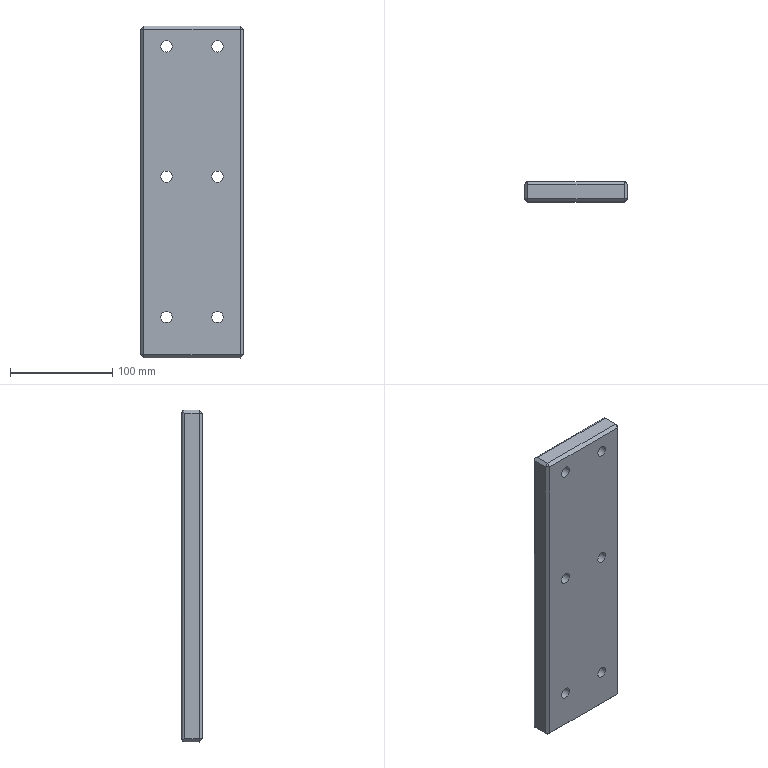Part | STEP file | lll_id1710_x_t | 1 solid | 40 faces | box 100 x 20 x 325 mm | volume 623377 mm3 | plane 24 | cylinder 16 | commonest cylinder face diameters 11 x6 17 x6 6 x4
STEP:
#1=CARTESIAN_POINT('',(2142.435,-593.,-282.5));
#2=VERTEX_POINT('',#1);
#3=CARTESIAN_POINT('',(2139.435,-593.,-285.5));
#4=VERTEX_POINT('',#3);
#5=CARTESIAN_POINT('',(2140.935,-593.,-284.));
#6=DIRECTION('',(-0.7071,0.000000065,-0.7071));
#7=VECTOR('',#6,1.);
#8=LINE('',#5,#7);
#9=EDGE_CURVE('',#2,#4,#8,.T.);
#10=ORIENTED_EDGE('',*,*,#9,.F.);
#11=CARTESIAN_POINT('',(2139.435,-596.,-282.5));
#12=VERTEX_POINT('',#11);
#13=CARTESIAN_POINT('',(2139.435,-596.,-282.5));
#14=DIRECTION('',(0.7071,0.7071,0.000000065));
#15=VECTOR('',#14,1.);
#16=LINE('',#13,#15);
#17=EDGE_CURVE('',#12,#2,#16,.T.);
#18=ORIENTED_EDGE('',*,*,#17,.F.);
#19=CARTESIAN_POINT('',(2139.435,-596.,-282.5));
#20=DIRECTION('',(0.,0.7071,-0.7071));
#21=VECTOR('',#20,1.);
#22=LINE('',#19,#21);
#23=EDGE_CURVE('',#12,#4,#22,.T.);
#24=ORIENTED_EDGE('',*,*,#23,.T.);
#25=EDGE_LOOP('',(#10,#18,#24));
#26=FACE_OUTER_BOUND('',#25,.T.);
#27=CARTESIAN_POINT('',(2139.435,-596.,-282.5));
#28=DIRECTION('',(0.5774,-0.5774,-0.5774));
#29=DIRECTION('',(0.,-0.7071,0.7071));
#30=AXIS2_PLACEMENT_3D('',#27,#28,#29);
#31=PLANE('',#30);
#32=ADVANCED_FACE('',(#26),#31,.T.);
#33=CARTESIAN_POINT('',(2142.435,-593.,36.5));
#34=VERTEX_POINT('',#33);
#35=CARTESIAN_POINT('',(2139.435,-596.,36.5));
#36=VERTEX_POINT('',#35);
#37=CARTESIAN_POINT('',(2142.435,-593.,36.5));
#38=DIRECTION('',(-0.7071,-0.7071,-0.000000065));
#39=VECTOR('',#38,1.);
#40=LINE('',#37,#39);
#41=EDGE_CURVE('',#34,#36,#40,.T.);
#42=ORIENTED_EDGE('',*,*,#41,.F.);
#43=CARTESIAN_POINT('',(2139.435,-593.,39.5));
#44=VERTEX_POINT('',#43);
#45=CARTESIAN_POINT('',(2142.435,-593.,36.5));
#46=DIRECTION('',(0.7071,0.000000065,-0.7071));
#47=VECTOR('',#46,1.);
#48=LINE('',#45,#47);
#49=EDGE_CURVE('',#44,#34,#48,.T.);
#50=ORIENTED_EDGE('',*,*,#49,.F.);
#51=CARTESIAN_POINT('',(2139.435,-594.5,38.));
#52=DIRECTION('',(0.,-0.7071,-0.7071));
#53=VECTOR('',#52,1.);
#54=LINE('',#51,#53);
#55=EDGE_CURVE('',#44,#36,#54,.T.);
#56=ORIENTED_EDGE('',*,*,#55,.T.);
#57=EDGE_LOOP('',(#42,#50,#56));
#58=FACE_OUTER_BOUND('',#57,.T.);
#59=CARTESIAN_POINT('',(2142.435,-593.,36.5));
#60=DIRECTION('',(0.5774,-0.5774,0.5774));
#61=DIRECTION('',(0.,0.7071,0.7071));
#62=AXIS2_PLACEMENT_3D('',#59,#60,#61);
#63=PLANE('',#62);
#64=ADVANCED_FACE('',(#58),#63,.T.);
#65=CARTESIAN_POINT('',(2045.435,-593.,-285.5));
#66=VERTEX_POINT('',#65);
#67=CARTESIAN_POINT('',(2042.435,-593.,-282.5));
#68=VERTEX_POINT('',#67);
#69=CARTESIAN_POINT('',(2043.935,-593.,-284.));
#70=DIRECTION('',(-0.7071,-0.000000065,0.7071));
#71=VECTOR('',#70,1.);
#72=LINE('',#69,#71);
#73=EDGE_CURVE('',#66,#68,#72,.T.);
#74=ORIENTED_EDGE('',*,*,#73,.F.);
#75=CARTESIAN_POINT('',(2045.435,-596.,-282.5));
#76=VERTEX_POINT('',#75);
#77=CARTESIAN_POINT('',(2045.435,-596.,-282.5));
#78=DIRECTION('',(0.,0.7071,-0.7071));
#79=VECTOR('',#78,1.);
#80=LINE('',#77,#79);
#81=EDGE_CURVE('',#76,#66,#80,.T.);
#82=ORIENTED_EDGE('',*,*,#81,.F.);
#83=CARTESIAN_POINT('',(2045.435,-596.,-282.5));
#84=DIRECTION('',(-0.7071,0.7071,0.000000065));
#85=VECTOR('',#84,1.);
#86=LINE('',#83,#85);
#87=EDGE_CURVE('',#76,#68,#86,.T.);
#88=ORIENTED_EDGE('',*,*,#87,.T.);
#89=EDGE_LOOP('',(#74,#82,#88));
#90=FACE_OUTER_BOUND('',#89,.T.);
#91=CARTESIAN_POINT('',(2045.435,-596.,-282.5));
#92=DIRECTION('',(-0.5774,-0.5774,-0.5774));
#93=DIRECTION('',(0.7071,0.000000065,-0.7071));
#94=AXIS2_PLACEMENT_3D('',#91,#92,#93);
#95=PLANE('',#94);
#96=ADVANCED_FACE('',(#90),#95,.T.);
#97=CARTESIAN_POINT('',(2045.435,-593.,39.5));
#98=VERTEX_POINT('',#97);
#99=CARTESIAN_POINT('',(2045.435,-596.,36.5));
#100=VERTEX_POINT('',#99);
#101=CARTESIAN_POINT('',(2045.435,-594.5,38.));
#102=DIRECTION('',(0.,-0.7071,-0.7071));
#103=VECTOR('',#102,1.);
#104=LINE('',#101,#103);
#105=EDGE_CURVE('',#98,#100,#104,.T.);
#106=ORIENTED_EDGE('',*,*,#105,.F.);
#107=CARTESIAN_POINT('',(2042.435,-593.,36.5));
#108=VERTEX_POINT('',#107);
#109=CARTESIAN_POINT('',(2042.435,-593.,36.5));
#110=DIRECTION('',(0.7071,-0.000000065,0.7071));
#111=VECTOR('',#110,1.);
#112=LINE('',#109,#111);
#113=EDGE_CURVE('',#108,#98,#112,.T.);
#114=ORIENTED_EDGE('',*,*,#113,.F.);
#115=CARTESIAN_POINT('',(2045.435,-596.,36.5));
#116=DIRECTION('',(0.7071,-0.7071,-0.000000065));
#117=VECTOR('',#116,1.);
#118=LINE('',#115,#117);
#119=EDGE_CURVE('',#108,#100,#118,.T.);
#120=ORIENTED_EDGE('',*,*,#119,.T.);
#121=EDGE_LOOP('',(#106,#114,#120));
#122=FACE_OUTER_BOUND('',#121,.T.);
#123=CARTESIAN_POINT('',(2042.435,-593.,36.5));
#124=DIRECTION('',(-0.5774,-0.5774,0.5774));
#125=DIRECTION('',(-0.7071,0.000000065,-0.7071));
#126=AXIS2_PLACEMENT_3D('',#123,#124,#125);
#127=PLANE('',#126);
#128=ADVANCED_FACE('',(#122),#127,.T.);
#129=CARTESIAN_POINT('',(2139.435,-579.,-285.5));
#130=VERTEX_POINT('',#129);
#131=CARTESIAN_POINT('',(2045.435,-579.,-285.5));
#132=VERTEX_POINT('',#131);
#133=CARTESIAN_POINT('',(2068.435,-579.,-285.5));
#134=DIRECTION('',(-1.,0.,0.));
#135=VECTOR('',#134,1.);
#136=LINE('',#133,#135);
#137=EDGE_CURVE('',#130,#132,#136,.T.);
#138=ORIENTED_EDGE('',*,*,#137,.F.);
#139=CARTESIAN_POINT('',(2139.435,-576.,-285.5));
#140=DIRECTION('',(0.,1.,0.000000092));
#141=VECTOR('',#140,1.);
#142=LINE('',#139,#141);
#143=EDGE_CURVE('',#4,#130,#142,.T.);
#144=ORIENTED_EDGE('',*,*,#143,.F.);
#145=CARTESIAN_POINT('',(2068.435,-593.,-285.5));
#146=DIRECTION('',(1.,0.,0.));
#147=VECTOR('',#146,1.);
#148=LINE('',#145,#147);
#149=EDGE_CURVE('',#66,#4,#148,.T.);
#150=ORIENTED_EDGE('',*,*,#149,.F.);
#151=CARTESIAN_POINT('',(2045.435,-576.,-285.5));
#152=DIRECTION('',(0.,-1.,-0.000000092));
#153=VECTOR('',#152,1.);
#154=LINE('',#151,#153);
#155=EDGE_CURVE('',#132,#66,#154,.T.);
#156=ORIENTED_EDGE('',*,*,#155,.F.);
#157=EDGE_LOOP('',(#138,#144,#150,#156));
#158=FACE_OUTER_BOUND('',#157,.T.);
#159=CARTESIAN_POINT('',(2068.435,-576.,-285.5));
#160=DIRECTION('',(0.,-0.000000092,1.));
#161=DIRECTION('',(0.,-1.,-0.000000092));
#162=AXIS2_PLACEMENT_3D('',#159,#160,#161);
#163=PLANE('',#162);
#164=ADVANCED_FACE('',(#158),#163,.F.);
#165=CARTESIAN_POINT('',(2043.935,-576.402,-284.));
#166=VERTEX_POINT('',#165);
#167=CARTESIAN_POINT('',(2042.435,-579.,-282.5));
#168=DIRECTION('',(-0.7071,0.000000065,-0.7071));
#169=DIRECTION('',(-0.7071,-0.000000065,0.7071));
#170=AXIS2_PLACEMENT_3D('',#167,#168,#169);
#171=ELLIPSE('',#170,4.243,3.);
#172=EDGE_CURVE('',#166,#132,#171,.T.);
#173=ORIENTED_EDGE('',*,*,#172,.T.);
#174=ORIENTED_EDGE('',*,*,#155,.T.);
#175=ORIENTED_EDGE('',*,*,#73,.T.);
#176=CARTESIAN_POINT('',(2042.435,-579.,-282.5));
#177=VERTEX_POINT('',#176);
#178=CARTESIAN_POINT('',(2042.435,-576.,-282.5));
#179=DIRECTION('',(0.,1.,0.000000092));
#180=VECTOR('',#179,1.);
#181=LINE('',#178,#180);
#182=EDGE_CURVE('',#68,#177,#181,.T.);
#183=ORIENTED_EDGE('',*,*,#182,.T.);
#184=CARTESIAN_POINT('',(2045.435,-579.,-285.5));
#185=DIRECTION('',(-0.7071,0.000000065,-0.7071));
#186=DIRECTION('',(-0.7071,0.000000016,0.7071));
#187=AXIS2_PLACEMENT_3D('',#184,#185,#186);
#188=ELLIPSE('',#187,4.243,3.);
#189=EDGE_CURVE('',#177,#166,#188,.T.);
#190=ORIENTED_EDGE('',*,*,#189,.T.);
#191=EDGE_LOOP('',(#173,#174,#175,#183,#190));
#192=FACE_OUTER_BOUND('',#191,.T.);
#193=CARTESIAN_POINT('',(2042.435,-576.,-282.5));
#194=DIRECTION('',(0.7071,-0.000000065,0.7071));
#195=DIRECTION('',(-0.7071,-0.000000065,0.7071));
#196=AXIS2_PLACEMENT_3D('',#193,#194,#195);
#197=PLANE('',#196);
#198=ADVANCED_FACE('',(#192),#197,.F.);
#199=CARTESIAN_POINT('',(2042.435,-579.,36.5));
#200=VERTEX_POINT('',#199);
#201=CARTESIAN_POINT('',(2042.435,-579.,-55.5));
#202=DIRECTION('',(0.,-0.000000035,1.));
#203=VECTOR('',#202,1.);
#204=LINE('',#201,#203);
#205=EDGE_CURVE('',#177,#200,#204,.T.);
#206=ORIENTED_EDGE('',*,*,#205,.F.);
#207=ORIENTED_EDGE('',*,*,#182,.F.);
#208=CARTESIAN_POINT('',(2042.435,-593.,69.5));
#209=DIRECTION('',(0.,0.000000092,-1.));
#210=VECTOR('',#209,1.);
#211=LINE('',#208,#210);
#212=EDGE_CURVE('',#108,#68,#211,.T.);
#213=ORIENTED_EDGE('',*,*,#212,.F.);
#214=CARTESIAN_POINT('',(2042.435,-576.,36.5));
#215=DIRECTION('',(0.,-1.,-0.000000092));
#216=VECTOR('',#215,1.);
#217=LINE('',#214,#216);
#218=EDGE_CURVE('',#200,#108,#217,.T.);
#219=ORIENTED_EDGE('',*,*,#218,.F.);
#220=EDGE_LOOP('',(#206,#207,#213,#219));
#221=FACE_OUTER_BOUND('',#220,.T.);
#222=CARTESIAN_POINT('',(2042.435,-576.,69.5));
#223=DIRECTION('',(1.,0.,0.));
#224=DIRECTION('',(0.,0.000000092,-1.));
#225=AXIS2_PLACEMENT_3D('',#222,#223,#224);
#226=PLANE('',#225);
#227=ADVANCED_FACE('',(#221),#226,.F.);
#228=CARTESIAN_POINT('',(2043.935,-576.402,38.));
#229=VERTEX_POINT('',#228);
#230=CARTESIAN_POINT('',(2045.435,-579.,39.5));
#231=DIRECTION('',(-0.7071,-0.000000062,0.7071));
#232=DIRECTION('',(0.7071,0.000000013,0.7071));
#233=AXIS2_PLACEMENT_3D('',#230,#231,#232);
#234=ELLIPSE('',#233,4.243,3.);
#235=EDGE_CURVE('',#229,#200,#234,.T.);
#236=ORIENTED_EDGE('',*,*,#235,.T.);
#237=ORIENTED_EDGE('',*,*,#218,.T.);
#238=ORIENTED_EDGE('',*,*,#113,.T.);
#239=CARTESIAN_POINT('',(2045.435,-579.,39.5));
#240=VERTEX_POINT('',#239);
#241=CARTESIAN_POINT('',(2045.435,-576.,39.5));
#242=DIRECTION('',(0.,1.,0.000000092));
#243=VECTOR('',#242,1.);
#244=LINE('',#241,#243);
#245=EDGE_CURVE('',#98,#240,#244,.T.);
#246=ORIENTED_EDGE('',*,*,#245,.T.);
#247=CARTESIAN_POINT('',(2042.435,-579.,36.5));
#248=DIRECTION('',(-0.7071,-0.000000065,0.7071));
#249=DIRECTION('',(-0.7071,0.000000065,-0.7071));
#250=AXIS2_PLACEMENT_3D('',#247,#248,#249);
#251=ELLIPSE('',#250,4.243,3.);
#252=EDGE_CURVE('',#240,#229,#251,.T.);
#253=ORIENTED_EDGE('',*,*,#252,.T.);
#254=EDGE_LOOP('',(#236,#237,#238,#246,#253));
#255=FACE_OUTER_BOUND('',#254,.T.);
#256=CARTESIAN_POINT('',(2045.435,-576.,39.5));
#257=DIRECTION('',(0.7071,0.000000065,-0.7071));
#258=DIRECTION('',(0.7071,-0.000000065,0.7071));
#259=AXIS2_PLACEMENT_3D('',#256,#257,#258);
#260=PLANE('',#259);
#261=ADVANCED_FACE('',(#255),#260,.F.);
#262=CARTESIAN_POINT('',(2116.435,-593.,39.5));
#263=DIRECTION('',(-1.,0.,0.));
#264=VECTOR('',#263,1.);
#265=LINE('',#262,#264);
#266=EDGE_CURVE('',#44,#98,#265,.T.);
#267=ORIENTED_EDGE('',*,*,#266,.F.);
#268=CARTESIAN_POINT('',(2139.435,-579.,39.5));
#269=VERTEX_POINT('',#268);
#270=CARTESIAN_POINT('',(2139.435,-576.,39.5));
#271=DIRECTION('',(0.,-1.,-0.000000092));
#272=VECTOR('',#271,1.);
#273=LINE('',#270,#272);
#274=EDGE_CURVE('',#269,#44,#273,.T.);
#275=ORIENTED_EDGE('',*,*,#274,.F.);
#276=CARTESIAN_POINT('',(2116.435,-579.,39.5));
#277=DIRECTION('',(1.,0.,0.));
#278=VECTOR('',#277,1.);
#279=LINE('',#276,#278);
#280=EDGE_CURVE('',#240,#269,#279,.T.);
#281=ORIENTED_EDGE('',*,*,#280,.F.);
#282=ORIENTED_EDGE('',*,*,#245,.F.);
#283=EDGE_LOOP('',(#267,#275,#281,#282));
#284=FACE_OUTER_BOUND('',#283,.T.);
#285=CARTESIAN_POINT('',(2116.435,-576.,39.5));
#286=DIRECTION('',(0.,0.000000092,-1.));
#287=DIRECTION('',(0.,1.,0.000000092));
#288=AXIS2_PLACEMENT_3D('',#285,#286,#287);
#289=PLANE('',#288);
#290=ADVANCED_FACE('',(#284),#289,.F.);
#291=CARTESIAN_POINT('',(2140.935,-576.402,-284.));
#292=VERTEX_POINT('',#291);
#293=CARTESIAN_POINT('',(2142.435,-579.,-282.5));
#294=VERTEX_POINT('',#293);
#295=CARTESIAN_POINT('',(2139.435,-579.,-285.5));
#296=DIRECTION('',(0.7071,0.000000065,-0.7071));
#297=DIRECTION('',(-0.7071,-0.000000016,-0.7071));
#298=AXIS2_PLACEMENT_3D('',#295,#296,#297);
#299=ELLIPSE('',#298,4.243,3.);
#300=EDGE_CURVE('',#292,#294,#299,.T.);
#301=ORIENTED_EDGE('',*,*,#300,.T.);
#302=CARTESIAN_POINT('',(2142.435,-576.,-282.5));
#303=DIRECTION('',(0.,-1.,-0.000000092));
#304=VECTOR('',#303,1.);
#305=LINE('',#302,#304);
#306=EDGE_CURVE('',#294,#2,#305,.T.);
#307=ORIENTED_EDGE('',*,*,#306,.T.);
#308=ORIENTED_EDGE('',*,*,#9,.T.);
#309=ORIENTED_EDGE('',*,*,#143,.T.);
#310=CARTESIAN_POINT('',(2142.435,-579.,-282.5));
#311=DIRECTION('',(0.7071,0.000000065,-0.7071));
#312=DIRECTION('',(-0.7071,0.000000065,-0.7071));
#313=AXIS2_PLACEMENT_3D('',#310,#311,#312);
#314=ELLIPSE('',#313,4.243,3.);
#315=EDGE_CURVE('',#130,#292,#314,.T.);
#316=ORIENTED_EDGE('',*,*,#315,.T.);
#317=EDGE_LOOP('',(#301,#307,#308,#309,#316));
#318=FACE_OUTER_BOUND('',#317,.T.);
#319=CARTESIAN_POINT('',(2139.435,-576.,-285.5));
#320=DIRECTION('',(-0.7071,-0.000000065,0.7071));
#321=DIRECTION('',(-0.7071,0.000000065,-0.7071));
#322=AXIS2_PLACEMENT_3D('',#319,#320,#321);
#323=PLANE('',#322);
#324=ADVANCED_FACE('',(#318),#323,.F.);
#325=CARTESIAN_POINT('',(2140.935,-576.402,38.));
#326=VERTEX_POINT('',#325);
#327=CARTESIAN_POINT('',(2142.435,-579.,36.5));
#328=DIRECTION('',(0.7071,-0.000000065,0.7071));
#329=DIRECTION('',(-0.7071,-0.000000065,0.7071));
#330=AXIS2_PLACEMENT_3D('',#327,#328,#329);
#331=ELLIPSE('',#330,4.243,3.);
#332=EDGE_CURVE('',#326,#269,#331,.T.);
#333=ORIENTED_EDGE('',*,*,#332,.T.);
#334=ORIENTED_EDGE('',*,*,#274,.T.);
#335=ORIENTED_EDGE('',*,*,#49,.T.);
#336=CARTESIAN_POINT('',(2142.435,-579.,36.5));
#337=VERTEX_POINT('',#336);
#338=CARTESIAN_POINT('',(2142.435,-576.,36.5));
#339=DIRECTION('',(0.,1.,0.000000092));
#340=VECTOR('',#339,1.);
#341=LINE('',#338,#340);
#342=EDGE_CURVE('',#34,#337,#341,.T.);
#343=ORIENTED_EDGE('',*,*,#342,.T.);
#344=CARTESIAN_POINT('',(2139.435,-579.,39.5));
#345=DIRECTION('',(0.7071,-0.000000062,0.7071));
#346=DIRECTION('',(0.7071,-0.000000013,-0.7071));
#347=AXIS2_PLACEMENT_3D('',#344,#345,#346);
#348=ELLIPSE('',#347,4.243,3.);
#349=EDGE_CURVE('',#337,#326,#348,.T.);
#350=ORIENTED_EDGE('',*,*,#349,.T.);
#351=EDGE_LOOP('',(#333,#334,#335,#343,#350));
#352=FACE_OUTER_BOUND('',#351,.T.);
#353=CARTESIAN_POINT('',(2142.435,-576.,36.5));
#354=DIRECTION('',(-0.7071,0.000000065,-0.7071));
#355=DIRECTION('',(0.7071,0.000000065,-0.7071));
#356=AXIS2_PLACEMENT_3D('',#353,#354,#355);
#357=PLANE('',#356);
#358=ADVANCED_FACE('',(#352),#357,.F.);
#359=CARTESIAN_POINT('',(2142.435,-593.,-55.5));
#360=DIRECTION('',(0.,-0.000000092,1.));
#361=VECTOR('',#360,1.);
#362=LINE('',#359,#361);
#363=EDGE_CURVE('',#2,#34,#362,.T.);
#364=ORIENTED_EDGE('',*,*,#363,.F.);
#365=ORIENTED_EDGE('',*,*,#306,.F.);
#366=CARTESIAN_POINT('',(2142.435,-579.,69.5));
#367=DIRECTION('',(0.,0.000000035,-1.));
#368=VECTOR('',#367,1.);
#369=LINE('',#366,#368);
#370=EDGE_CURVE('',#337,#294,#369,.T.);
#371=ORIENTED_EDGE('',*,*,#370,.F.);
#372=ORIENTED_EDGE('',*,*,#342,.F.);
#373=EDGE_LOOP('',(#364,#365,#371,#372));
#374=FACE_OUTER_BOUND('',#373,.T.);
#375=CARTESIAN_POINT('',(2142.435,-576.,-55.5));
#376=DIRECTION('',(-1.,0.,0.));
#377=DIRECTION('',(0.,-0.000000092,1.));
#378=AXIS2_PLACEMENT_3D('',#375,#376,#377);
#379=PLANE('',#378);
#380=ADVANCED_FACE('',(#374),#379,.F.);
#381=CARTESIAN_POINT('',(2117.435,-588.,-251.));
#382=VERTEX_POINT('',#381);
#383=CARTESIAN_POINT('',(2117.435,-588.,-245.5));
#384=DIRECTION('',(0.,-1.,-0.000000092));
#385=DIRECTION('',(0.,0.000000092,-1.));
#386=AXIS2_PLACEMENT_3D('',#383,#384,#385);
#387=CIRCLE('',#386,5.5);
#388=EDGE_CURVE('',#382,#382,#387,.T.);
#389=ORIENTED_EDGE('',*,*,#388,.T.);
#390=EDGE_LOOP('',(#389));
#391=FACE_BOUND('',#390,.T.);
#392=CARTESIAN_POINT('',(2117.435,-588.,-254.));
#393=VERTEX_POINT('',#392);
#394=CARTESIAN_POINT('',(2117.435,-588.,-245.5));
#395=DIRECTION('',(0.,-1.,-0.000000092));
#396=DIRECTION('',(0.,0.000000092,-1.));
#397=AXIS2_PLACEMENT_3D('',#394,#395,#396);
#398=CIRCLE('',#397,8.5);
#399=EDGE_CURVE('',#393,#393,#398,.T.);
#400=ORIENTED_EDGE('',*,*,#399,.F.);
#401=EDGE_LOOP('',(#400));
#402=FACE_BOUND('',#401,.T.);
#403=CARTESIAN_POINT('',(2117.435,-588.,-245.5));
#404=DIRECTION('',(0.,-1.,-0.000000092));
#405=DIRECTION('',(0.,0.000000092,-1.));
#406=AXIS2_PLACEMENT_3D('',#403,#404,#405);
#407=PLANE('',#406);
#408=ADVANCED_FACE('',(#391,#402),#407,.F.);
#409=CARTESIAN_POINT('',(2067.435,-588.,-251.));
#410=VERTEX_POINT('',#409);
#411=CARTESIAN_POINT('',(2067.435,-588.,-245.5));
#412=DIRECTION('',(0.,-1.,-0.000000092));
#413=DIRECTION('',(0.,0.000000092,-1.));
#414=AXIS2_PLACEMENT_3D('',#411,#412,#413);
#415=CIRCLE('',#414,5.5);
#416=EDGE_CURVE('',#410,#410,#415,.T.);
#417=ORIENTED_EDGE('',*,*,#416,.T.);
#418=EDGE_LOOP('',(#417));
#419=FACE_BOUND('',#418,.T.);
#420=CARTESIAN_POINT('',(2067.435,-588.,-254.));
#421=VERTEX_POINT('',#420);
#422=CARTESIAN_POINT('',(2067.435,-588.,-245.5));
#423=DIRECTION('',(0.,-1.,-0.000000092));
#424=DIRECTION('',(0.,0.000000092,-1.));
#425=AXIS2_PLACEMENT_3D('',#422,#423,#424);
#426=CIRCLE('',#425,8.5);
#427=EDGE_CURVE('',#421,#421,#426,.T.);
#428=ORIENTED_EDGE('',*,*,#427,.F.);
#429=EDGE_LOOP('',(#428));
#430=FACE_BOUND('',#429,.T.);
#431=CARTESIAN_POINT('',(2067.435,-588.,-245.5));
#432=DIRECTION('',(0.,-1.,-0.000000092));
#433=DIRECTION('',(0.,0.000000092,-1.));
#434=AXIS2_PLACEMENT_3D('',#431,#432,#433);
#435=PLANE('',#434);
#436=ADVANCED_FACE('',(#419,#430),#435,.F.);
#437=CARTESIAN_POINT('',(2067.435,-588.,25.));
#438=VERTEX_POINT('',#437);
#439=CARTESIAN_POINT('',(2067.435,-588.,19.5));
#440=DIRECTION('',(0.,-1.,-0.000000092));
#441=DIRECTION('',(0.,-0.000000092,1.));
#442=AXIS2_PLACEMENT_3D('',#439,#440,#441);
#443=CIRCLE('',#442,5.5);
#444=EDGE_CURVE('',#438,#438,#443,.T.);
#445=ORIENTED_EDGE('',*,*,#444,.T.);
#446=EDGE_LOOP('',(#445));
#447=FACE_BOUND('',#446,.T.);
#448=CARTESIAN_POINT('',(2067.435,-588.,28.));
#449=VERTEX_POINT('',#448);
#450=CARTESIAN_POINT('',(2067.435,-588.,19.5));
#451=DIRECTION('',(0.,-1.,-0.000000092));
#452=DIRECTION('',(0.,-0.000000092,1.));
#453=AXIS2_PLACEMENT_3D('',#450,#451,#452);
#454=CIRCLE('',#453,8.5);
#455=EDGE_CURVE('',#449,#449,#454,.T.);
#456=ORIENTED_EDGE('',*,*,#455,.F.);
#457=EDGE_LOOP('',(#456));
#458=FACE_BOUND('',#457,.T.);
#459=CARTESIAN_POINT('',(2067.435,-588.,19.5));
#460=DIRECTION('',(0.,-1.,-0.000000092));
#461=DIRECTION('',(0.,-0.000000092,1.));
#462=AXIS2_PLACEMENT_3D('',#459,#460,#461);
#463=PLANE('',#462);
#464=ADVANCED_FACE('',(#447,#458),#463,.F.);
#465=CARTESIAN_POINT('',(2117.435,-588.,25.));
#466=VERTEX_POINT('',#465);
#467=CARTESIAN_POINT('',(2117.435,-588.,19.5));
#468=DIRECTION('',(0.,-1.,-0.000000092));
#469=DIRECTION('',(0.,-0.000000092,1.));
#470=AXIS2_PLACEMENT_3D('',#467,#468,#469);
#471=CIRCLE('',#470,5.5);
#472=EDGE_CURVE('',#466,#466,#471,.T.);
#473=ORIENTED_EDGE('',*,*,#472,.T.);
#474=EDGE_LOOP('',(#473));
#475=FACE_BOUND('',#474,.T.);
#476=CARTESIAN_POINT('',(2117.435,-588.,28.));
#477=VERTEX_POINT('',#476);
#478=CARTESIAN_POINT('',(2117.435,-588.,19.5));
#479=DIRECTION('',(0.,-1.,-0.000000092));
#480=DIRECTION('',(0.,-0.000000092,1.));
#481=AXIS2_PLACEMENT_3D('',#478,#479,#480);
#482=CIRCLE('',#481,8.5);
#483=EDGE_CURVE('',#477,#477,#482,.T.);
#484=ORIENTED_EDGE('',*,*,#483,.F.);
#485=EDGE_LOOP('',(#484));
#486=FACE_BOUND('',#485,.T.);
#487=CARTESIAN_POINT('',(2117.435,-588.,19.5));
#488=DIRECTION('',(0.,-1.,-0.000000092));
#489=DIRECTION('',(0.,-0.000000092,1.));
#490=AXIS2_PLACEMENT_3D('',#487,#488,#489);
#491=PLANE('',#490);
#492=ADVANCED_FACE('',(#475,#486),#491,.F.);
#493=CARTESIAN_POINT('',(2139.435,-576.,-282.5));
#494=VERTEX_POINT('',#493);
#495=CARTESIAN_POINT('',(2139.435,-579.,-282.5));
#496=DIRECTION('',(0.7071,-0.000000025,0.7071));
#497=DIRECTION('',(-0.7071,-0.000000025,0.7071));
#498=AXIS2_PLACEMENT_3D('',#495,#496,#497);
#499=ELLIPSE('',#498,4.243,3.);
#500=EDGE_CURVE('',#292,#494,#499,.T.);
#501=ORIENTED_EDGE('',*,*,#500,.F.);
#502=ORIENTED_EDGE('',*,*,#315,.F.);
#503=ORIENTED_EDGE('',*,*,#137,.T.);
#504=ORIENTED_EDGE('',*,*,#172,.F.);
#505=CARTESIAN_POINT('',(2045.435,-576.,-282.5));
#506=VERTEX_POINT('',#505);
#507=CARTESIAN_POINT('',(2045.435,-579.,-282.5));
#508=DIRECTION('',(0.7071,0.000000025,-0.7071));
#509=DIRECTION('',(0.7071,-0.000000025,0.7071));
#510=AXIS2_PLACEMENT_3D('',#507,#508,#509);
#511=ELLIPSE('',#510,4.243,3.);
#512=EDGE_CURVE('',#166,#506,#511,.T.);
#513=ORIENTED_EDGE('',*,*,#512,.T.);
#514=CARTESIAN_POINT('',(2068.435,-576.,-282.5));
#515=DIRECTION('',(1.,0.,0.));
#516=VECTOR('',#515,1.);
#517=LINE('',#514,#516);
#518=EDGE_CURVE('',#506,#494,#517,.T.);
#519=ORIENTED_EDGE('',*,*,#518,.T.);
#520=EDGE_LOOP('',(#501,#502,#503,#504,#513,#519));
#521=FACE_OUTER_BOUND('',#520,.T.);
#522=CARTESIAN_POINT('',(2068.435,-579.,-282.5));
#523=DIRECTION('',(-1.,0.,0.));
#524=DIRECTION('',(0.,1.,0.));
#525=AXIS2_PLACEMENT_3D('',#522,#523,#524);
#526=CYLINDRICAL_SURFACE('',#525,3.);
#527=ADVANCED_FACE('',(#521),#526,.T.);
#528=CARTESIAN_POINT('',(2045.435,-576.,36.5));
#529=VERTEX_POINT('',#528);
#530=CARTESIAN_POINT('',(2045.435,-576.,69.5));
#531=DIRECTION('',(0.,0.000000035,-1.));
#532=VECTOR('',#531,1.);
#533=LINE('',#530,#532);
#534=EDGE_CURVE('',#529,#506,#533,.T.);
#535=ORIENTED_EDGE('',*,*,#534,.T.);
#536=ORIENTED_EDGE('',*,*,#512,.F.);
#537=ORIENTED_EDGE('',*,*,#189,.F.);
#538=ORIENTED_EDGE('',*,*,#205,.T.);
#539=ORIENTED_EDGE('',*,*,#235,.F.);
#540=CARTESIAN_POINT('',(2045.435,-579.,36.5));
#541=DIRECTION('',(0.7071,-0.000000025,0.7071));
#542=DIRECTION('',(-0.7071,-0.000000025,0.7071));
#543=AXIS2_PLACEMENT_3D('',#540,#541,#542);
#544=ELLIPSE('',#543,4.243,3.);
#545=EDGE_CURVE('',#529,#229,#544,.T.);
#546=ORIENTED_EDGE('',*,*,#545,.F.);
#547=EDGE_LOOP('',(#535,#536,#537,#538,#539,#546));
#548=FACE_OUTER_BOUND('',#547,.T.);
#549=CARTESIAN_POINT('',(2045.435,-579.,69.5));
#550=DIRECTION('',(0.,-0.000000035,1.));
#551=DIRECTION('',(-1.,0.,0.));
#552=AXIS2_PLACEMENT_3D('',#549,#550,#551);
#553=CYLINDRICAL_SURFACE('',#552,3.);
#554=ADVANCED_FACE('',(#548),#553,.T.);
#555=ORIENTED_EDGE('',*,*,#280,.T.);
#556=ORIENTED_EDGE('',*,*,#332,.F.);
#557=CARTESIAN_POINT('',(2139.435,-576.,36.5));
#558=VERTEX_POINT('',#557);
#559=CARTESIAN_POINT('',(2139.435,-579.,36.5));
#560=DIRECTION('',(-0.7071,-0.000000025,0.7071));
#561=DIRECTION('',(-0.7071,0.000000025,-0.7071));
#562=AXIS2_PLACEMENT_3D('',#559,#560,#561);
#563=ELLIPSE('',#562,4.243,3.);
#564=EDGE_CURVE('',#326,#558,#563,.T.);
#565=ORIENTED_EDGE('',*,*,#564,.T.);
#566=CARTESIAN_POINT('',(2116.435,-576.,36.5));
#567=DIRECTION('',(-1.,0.,0.));
#568=VECTOR('',#567,1.);
#569=LINE('',#566,#568);
#570=EDGE_CURVE('',#558,#529,#569,.T.);
#571=ORIENTED_EDGE('',*,*,#570,.T.);
#572=ORIENTED_EDGE('',*,*,#545,.T.);
#573=ORIENTED_EDGE('',*,*,#252,.F.);
#574=EDGE_LOOP('',(#555,#556,#565,#571,#572,#573));
#575=FACE_OUTER_BOUND('',#574,.T.);
#576=CARTESIAN_POINT('',(2116.435,-579.,36.5));
#577=DIRECTION('',(-1.,0.,0.));
#578=DIRECTION('',(0.,1.,0.));
#579=AXIS2_PLACEMENT_3D('',#576,#577,#578);
#580=CYLINDRICAL_SURFACE('',#579,3.);
#581=ADVANCED_FACE('',(#575),#580,.T.);
#582=ORIENTED_EDGE('',*,*,#370,.T.);
#583=ORIENTED_EDGE('',*,*,#300,.F.);
#584=ORIENTED_EDGE('',*,*,#500,.T.);
#585=CARTESIAN_POINT('',(2139.435,-576.,-55.5));
#586=DIRECTION('',(0.,-0.000000035,1.));
#587=VECTOR('',#586,1.);
#588=LINE('',#585,#587);
#589=EDGE_CURVE('',#494,#558,#588,.T.);
#590=ORIENTED_EDGE('',*,*,#589,.T.);
#591=ORIENTED_EDGE('',*,*,#564,.F.);
#592=ORIENTED_EDGE('',*,*,#349,.F.);
#593=EDGE_LOOP('',(#582,#583,#584,#590,#591,#592));
#594=FACE_OUTER_BOUND('',#593,.T.);
#595=CARTESIAN_POINT('',(2139.435,-579.,-55.5));
#596=DIRECTION('',(0.,0.000000035,-1.));
#597=DIRECTION('',(1.,0.,0.));
#598=AXIS2_PLACEMENT_3D('',#595,#596,#597);
#599=CYLINDRICAL_SURFACE('',#598,3.);
#600=ADVANCED_FACE('',(#594),#599,.T.);
#601=ORIENTED_EDGE('',*,*,#399,.T.);
#602=EDGE_LOOP('',(#601));
#603=FACE_BOUND('',#602,.T.);
#604=CARTESIAN_POINT('',(2117.435,-576.,-254.));
#605=VERTEX_POINT('',#604);
#606=CARTESIAN_POINT('',(2117.435,-576.,-245.5));
#607=DIRECTION('',(0.,-1.,-0.000000035));
#608=DIRECTION('',(0.,0.000000035,-1.));
#609=AXIS2_PLACEMENT_3D('',#606,#607,#608);
#610=CIRCLE('',#609,8.5);
#611=EDGE_CURVE('',#605,#605,#610,.T.);
#612=ORIENTED_EDGE('',*,*,#611,.F.);
#613=EDGE_LOOP('',(#612));
#614=FACE_BOUND('',#613,.T.);
#615=CARTESIAN_POINT('',(2117.435,-576.,-245.5));
#616=DIRECTION('',(0.,-1.,-0.000000092));
#617=DIRECTION('',(0.,0.000000092,-1.));
#618=AXIS2_PLACEMENT_3D('',#615,#616,#617);
#619=CYLINDRICAL_SURFACE('',#618,8.5);
#620=ADVANCED_FACE('',(#603,#614),#619,.F.);
#621=ORIENTED_EDGE('',*,*,#427,.T.);
#622=EDGE_LOOP('',(#621));
#623=FACE_BOUND('',#622,.T.);
#624=CARTESIAN_POINT('',(2067.435,-576.,-254.));
#625=VERTEX_POINT('',#624);
#626=CARTESIAN_POINT('',(2067.435,-576.,-245.5));
#627=DIRECTION('',(0.,-1.,-0.000000035));
#628=DIRECTION('',(0.,0.000000035,-1.));
#629=AXIS2_PLACEMENT_3D('',#626,#627,#628);
#630=CIRCLE('',#629,8.5);
#631=EDGE_CURVE('',#625,#625,#630,.T.);
#632=ORIENTED_EDGE('',*,*,#631,.F.);
#633=EDGE_LOOP('',(#632));
#634=FACE_BOUND('',#633,.T.);
#635=CARTESIAN_POINT('',(2067.435,-576.,-245.5));
#636=DIRECTION('',(0.,-1.,-0.000000092));
#637=DIRECTION('',(0.,0.000000092,-1.));
#638=AXIS2_PLACEMENT_3D('',#635,#636,#637);
#639=CYLINDRICAL_SURFACE('',#638,8.5);
#640=ADVANCED_FACE('',(#623,#634),#639,.F.);
#641=CARTESIAN_POINT('',(2067.435,-576.,11.));
#642=VERTEX_POINT('',#641);
#643=CARTESIAN_POINT('',(2067.435,-576.,19.5));
#644=DIRECTION('',(0.,-1.,-0.000000035));
#645=DIRECTION('',(0.,0.000000035,-1.));
#646=AXIS2_PLACEMENT_3D('',#643,#644,#645);
#647=CIRCLE('',#646,8.5);
#648=EDGE_CURVE('',#642,#642,#647,.T.);
#649=ORIENTED_EDGE('',*,*,#648,.F.);
#650=EDGE_LOOP('',(#649));
#651=FACE_BOUND('',#650,.T.);
#652=ORIENTED_EDGE('',*,*,#455,.T.);
#653=EDGE_LOOP('',(#652));
#654=FACE_BOUND('',#653,.T.);
#655=CARTESIAN_POINT('',(2067.435,-576.,19.5));
#656=DIRECTION('',(0.,-1.,-0.000000092));
#657=DIRECTION('',(0.,-0.000000092,1.));
#658=AXIS2_PLACEMENT_3D('',#655,#656,#657);
#659=CYLINDRICAL_SURFACE('',#658,8.5);
#660=ADVANCED_FACE('',(#651,#654),#659,.F.);
#661=CARTESIAN_POINT('',(2117.435,-576.,11.));
#662=VERTEX_POINT('',#661);
#663=CARTESIAN_POINT('',(2117.435,-576.,19.5));
#664=DIRECTION('',(0.,-1.,-0.000000035));
#665=DIRECTION('',(0.,0.000000035,-1.));
#666=AXIS2_PLACEMENT_3D('',#663,#664,#665);
#667=CIRCLE('',#666,8.5);
#668=EDGE_CURVE('',#662,#662,#667,.T.);
#669=ORIENTED_EDGE('',*,*,#668,.F.);
#670=EDGE_LOOP('',(#669));
#671=FACE_BOUND('',#670,.T.);
#672=ORIENTED_EDGE('',*,*,#483,.T.);
#673=EDGE_LOOP('',(#672));
#674=FACE_BOUND('',#673,.T.);
#675=CARTESIAN_POINT('',(2117.435,-576.,19.5));
#676=DIRECTION('',(0.,-1.,-0.000000092));
#677=DIRECTION('',(0.,-0.000000092,1.));
#678=AXIS2_PLACEMENT_3D('',#675,#676,#677);
#679=CYLINDRICAL_SURFACE('',#678,8.5);
#680=ADVANCED_FACE('',(#671,#674),#679,.F.);
#681=CARTESIAN_POINT('',(2117.435,-576.,-116.5));
#682=VERTEX_POINT('',#681);
#683=CARTESIAN_POINT('',(2117.435,-576.,-108.));
#684=DIRECTION('',(0.,-1.,-0.000000035));
#685=DIRECTION('',(0.,0.000000035,-1.));
#686=AXIS2_PLACEMENT_3D('',#683,#684,#685);
#687=CIRCLE('',#686,8.5);
#688=EDGE_CURVE('',#682,#682,#687,.T.);
#689=ORIENTED_EDGE('',*,*,#688,.T.);
#690=EDGE_LOOP('',(#689));
#691=FACE_BOUND('',#690,.T.);
#692=CARTESIAN_POINT('',(2067.435,-576.,-116.5));
#693=VERTEX_POINT('',#692);
#694=CARTESIAN_POINT('',(2067.435,-576.,-108.));
#695=DIRECTION('',(0.,-1.,-0.000000035));
#696=DIRECTION('',(0.,0.000000035,-1.));
#697=AXIS2_PLACEMENT_3D('',#694,#695,#696);
#698=CIRCLE('',#697,8.5);
#699=EDGE_CURVE('',#693,#693,#698,.T.);
#700=ORIENTED_EDGE('',*,*,#699,.T.);
#701=EDGE_LOOP('',(#700));
#702=FACE_BOUND('',#701,.T.);
#703=ORIENTED_EDGE('',*,*,#668,.T.);
#704=EDGE_LOOP('',(#703));
#705=FACE_BOUND('',#704,.T.);
#706=ORIENTED_EDGE('',*,*,#648,.T.);
#707=EDGE_LOOP('',(#706));
#708=FACE_BOUND('',#707,.T.);
#709=ORIENTED_EDGE('',*,*,#631,.T.);
#710=EDGE_LOOP('',(#709));
#711=FACE_BOUND('',#710,.T.);
#712=ORIENTED_EDGE('',*,*,#611,.T.);
#713=EDGE_LOOP('',(#712));
#714=FACE_BOUND('',#713,.T.);
#715=ORIENTED_EDGE('',*,*,#589,.F.);
#716=ORIENTED_EDGE('',*,*,#518,.F.);
#717=ORIENTED_EDGE('',*,*,#534,.F.);
#718=ORIENTED_EDGE('',*,*,#570,.F.);
#719=EDGE_LOOP('',(#715,#716,#717,#718));
#720=FACE_BOUND('',#719,.T.);
#721=CARTESIAN_POINT('',(2068.435,-576.,-55.5));
#722=DIRECTION('',(0.,1.,0.000000035));
#723=DIRECTION('',(0.,-0.000000035,1.));
#724=AXIS2_PLACEMENT_3D('',#721,#722,#723);
#725=PLANE('',#724);
#726=ADVANCED_FACE('',(#691,#702,#705,#708,#711,#714,#720),#725,.T.);
#727=ORIENTED_EDGE('',*,*,#23,.F.);
#728=CARTESIAN_POINT('',(2068.435,-596.,-282.5));
#729=DIRECTION('',(-1.,0.,0.));
#730=VECTOR('',#729,1.);
#731=LINE('',#728,#730);
#732=EDGE_CURVE('',#12,#76,#731,.T.);
#733=ORIENTED_EDGE('',*,*,#732,.T.);
#734=ORIENTED_EDGE('',*,*,#81,.T.);
#735=ORIENTED_EDGE('',*,*,#149,.T.);
#736=EDGE_LOOP('',(#727,#733,#734,#735));
#737=FACE_OUTER_BOUND('',#736,.T.);
#738=CARTESIAN_POINT('',(2068.435,-596.,-282.5));
#739=DIRECTION('',(0.,0.7071,0.7071));
#740=DIRECTION('',(0.,0.7071,-0.7071));
#741=AXIS2_PLACEMENT_3D('',#738,#739,#740);
#742=PLANE('',#741);
#743=ADVANCED_FACE('',(#737),#742,.F.);
#744=CARTESIAN_POINT('',(2139.435,-596.,-55.5));
#745=DIRECTION('',(0.,0.000000092,-1.));
#746=VECTOR('',#745,1.);
#747=LINE('',#744,#746);
#748=EDGE_CURVE('',#36,#12,#747,.T.);
#749=ORIENTED_EDGE('',*,*,#748,.T.);
#750=ORIENTED_EDGE('',*,*,#17,.T.);
#751=ORIENTED_EDGE('',*,*,#363,.T.);
#752=ORIENTED_EDGE('',*,*,#41,.T.);
#753=EDGE_LOOP('',(#749,#750,#751,#752));
#754=FACE_OUTER_BOUND('',#753,.T.);
#755=CARTESIAN_POINT('',(2139.435,-596.,-55.5));
#756=DIRECTION('',(-0.7071,0.7071,0.000000065));
#757=DIRECTION('',(-0.7071,-0.7071,-0.000000065));
#758=AXIS2_PLACEMENT_3D('',#755,#756,#757);
#759=PLANE('',#758);
#760=ADVANCED_FACE('',(#754),#759,.F.);
#761=ORIENTED_EDGE('',*,*,#55,.F.);
#762=ORIENTED_EDGE('',*,*,#266,.T.);
#763=ORIENTED_EDGE('',*,*,#105,.T.);
#764=CARTESIAN_POINT('',(2068.435,-596.,36.5));
#765=DIRECTION('',(1.,0.,0.));
#766=VECTOR('',#765,1.);
#767=LINE('',#764,#766);
#768=EDGE_CURVE('',#100,#36,#767,.T.);
#769=ORIENTED_EDGE('',*,*,#768,.T.);
#770=EDGE_LOOP('',(#761,#762,#763,#769));
#771=FACE_OUTER_BOUND('',#770,.T.);
#772=CARTESIAN_POINT('',(2068.435,-596.,36.5));
#773=DIRECTION('',(0.,0.7071,-0.7071));
#774=DIRECTION('',(0.,-0.7071,-0.7071));
#775=AXIS2_PLACEMENT_3D('',#772,#773,#774);
#776=PLANE('',#775);
#777=ADVANCED_FACE('',(#771),#776,.F.);
#778=ORIENTED_EDGE('',*,*,#212,.T.);
#779=ORIENTED_EDGE('',*,*,#87,.F.);
#780=CARTESIAN_POINT('',(2045.435,-596.,-55.5));
#781=DIRECTION('',(0.,-0.000000092,1.));
#782=VECTOR('',#781,1.);
#783=LINE('',#780,#782);
#784=EDGE_CURVE('',#76,#100,#783,.T.);
#785=ORIENTED_EDGE('',*,*,#784,.T.);
#786=ORIENTED_EDGE('',*,*,#119,.F.);
#787=EDGE_LOOP('',(#778,#779,#785,#786));
#788=FACE_OUTER_BOUND('',#787,.T.);
#789=CARTESIAN_POINT('',(2045.435,-596.,-55.5));
#790=DIRECTION('',(0.7071,0.7071,0.000000065));
#791=DIRECTION('',(-0.7071,0.7071,0.000000065));
#792=AXIS2_PLACEMENT_3D('',#789,#790,#791);
#793=PLANE('',#792);
#794=ADVANCED_FACE('',(#788),#793,.F.);
#795=ORIENTED_EDGE('',*,*,#388,.F.);
#796=EDGE_LOOP('',(#795));
#797=FACE_BOUND('',#796,.T.);
#798=CARTESIAN_POINT('',(2117.435,-596.,-240.));
#799=VERTEX_POINT('',#798);
#800=CARTESIAN_POINT('',(2117.435,-596.,-245.5));
#801=DIRECTION('',(0.,1.,0.000000092));
#802=DIRECTION('',(0.,-0.000000092,1.));
#803=AXIS2_PLACEMENT_3D('',#800,#801,#802);
#804=CIRCLE('',#803,5.5);
#805=EDGE_CURVE('',#799,#799,#804,.T.);
#806=ORIENTED_EDGE('',*,*,#805,.F.);
#807=EDGE_LOOP('',(#806));
#808=FACE_BOUND('',#807,.T.);
#809=CARTESIAN_POINT('',(2117.435,-636.,-245.5));
#810=DIRECTION('',(0.,-1.,-0.000000092));
#811=DIRECTION('',(0.,0.000000092,-1.));
#812=AXIS2_PLACEMENT_3D('',#809,#810,#811);
#813=CYLINDRICAL_SURFACE('',#812,5.5);
#814=ADVANCED_FACE('',(#797,#808),#813,.F.);
#815=ORIENTED_EDGE('',*,*,#416,.F.);
#816=EDGE_LOOP('',(#815));
#817=FACE_BOUND('',#816,.T.);
#818=CARTESIAN_POINT('',(2067.435,-596.,-251.));
#819=VERTEX_POINT('',#818);
#820=CARTESIAN_POINT('',(2067.435,-596.,-245.5));
#821=DIRECTION('',(0.,-1.,-0.000000092));
#822=DIRECTION('',(0.,0.000000092,-1.));
#823=AXIS2_PLACEMENT_3D('',#820,#821,#822);
#824=CIRCLE('',#823,5.5);
#825=EDGE_CURVE('',#819,#819,#824,.T.);
#826=ORIENTED_EDGE('',*,*,#825,.T.);
#827=EDGE_LOOP('',(#826));
#828=FACE_BOUND('',#827,.T.);
#829=CARTESIAN_POINT('',(2067.435,-636.,-245.5));
#830=DIRECTION('',(0.,-1.,-0.000000092));
#831=DIRECTION('',(0.,0.000000092,-1.));
#832=AXIS2_PLACEMENT_3D('',#829,#830,#831);
#833=CYLINDRICAL_SURFACE('',#832,5.5);
#834=ADVANCED_FACE('',(#817,#828),#833,.F.);
#835=ORIENTED_EDGE('',*,*,#444,.F.);
#836=EDGE_LOOP('',(#835));
#837=FACE_BOUND('',#836,.T.);
#838=CARTESIAN_POINT('',(2067.435,-596.,14.));
#839=VERTEX_POINT('',#838);
#840=CARTESIAN_POINT('',(2067.435,-596.,19.5));
#841=DIRECTION('',(0.,-1.,-0.000000092));
#842=DIRECTION('',(0.,0.000000092,-1.));
#843=AXIS2_PLACEMENT_3D('',#840,#841,#842);
#844=CIRCLE('',#843,5.5);
#845=EDGE_CURVE('',#839,#839,#844,.T.);
#846=ORIENTED_EDGE('',*,*,#845,.T.);
#847=EDGE_LOOP('',(#846));
#848=FACE_BOUND('',#847,.T.);
#849=CARTESIAN_POINT('',(2067.435,-636.,19.5));
#850=DIRECTION('',(0.,-1.,-0.000000092));
#851=DIRECTION('',(0.,-0.000000092,1.));
#852=AXIS2_PLACEMENT_3D('',#849,#850,#851);
#853=CYLINDRICAL_SURFACE('',#852,5.5);
#854=ADVANCED_FACE('',(#837,#848),#853,.F.);
#855=ORIENTED_EDGE('',*,*,#472,.F.);
#856=EDGE_LOOP('',(#855));
#857=FACE_BOUND('',#856,.T.);
#858=CARTESIAN_POINT('',(2117.435,-596.,14.));
#859=VERTEX_POINT('',#858);
#860=CARTESIAN_POINT('',(2117.435,-596.,19.5));
#861=DIRECTION('',(0.,-1.,-0.000000092));
#862=DIRECTION('',(0.,0.000000092,-1.));
#863=AXIS2_PLACEMENT_3D('',#860,#861,#862);
#864=CIRCLE('',#863,5.5);
#865=EDGE_CURVE('',#859,#859,#864,.T.);
#866=ORIENTED_EDGE('',*,*,#865,.T.);
#867=EDGE_LOOP('',(#866));
#868=FACE_BOUND('',#867,.T.);
#869=CARTESIAN_POINT('',(2117.435,-636.,19.5));
#870=DIRECTION('',(0.,-1.,-0.000000092));
#871=DIRECTION('',(0.,-0.000000092,1.));
#872=AXIS2_PLACEMENT_3D('',#869,#870,#871);
#873=CYLINDRICAL_SURFACE('',#872,5.5);
#874=ADVANCED_FACE('',(#857,#868),#873,.F.);
#875=CARTESIAN_POINT('',(2117.435,-596.,-113.5));
#876=VERTEX_POINT('',#875);
#877=CARTESIAN_POINT('',(2117.435,-596.,-108.));
#878=DIRECTION('',(0.,-1.,-0.000000092));
#879=DIRECTION('',(0.,0.000000092,-1.));
#880=AXIS2_PLACEMENT_3D('',#877,#878,#879);
#881=CIRCLE('',#880,5.5);
#882=EDGE_CURVE('',#876,#876,#881,.T.);
#883=ORIENTED_EDGE('',*,*,#882,.F.);
#884=EDGE_LOOP('',(#883));
#885=FACE_BOUND('',#884,.T.);
#886=CARTESIAN_POINT('',(2067.435,-596.,-113.5));
#887=VERTEX_POINT('',#886);
#888=CARTESIAN_POINT('',(2067.435,-596.,-108.));
#889=DIRECTION('',(0.,-1.,-0.000000092));
#890=DIRECTION('',(0.,0.000000092,-1.));
#891=AXIS2_PLACEMENT_3D('',#888,#889,#890);
#892=CIRCLE('',#891,5.5);
#893=EDGE_CURVE('',#887,#887,#892,.T.);
#894=ORIENTED_EDGE('',*,*,#893,.F.);
#895=EDGE_LOOP('',(#894));
#896=FACE_BOUND('',#895,.T.);
#897=ORIENTED_EDGE('',*,*,#865,.F.);
#898=EDGE_LOOP('',(#897));
#899=FACE_BOUND('',#898,.T.);
#900=ORIENTED_EDGE('',*,*,#845,.F.);
#901=EDGE_LOOP('',(#900));
#902=FACE_BOUND('',#901,.T.);
#903=ORIENTED_EDGE('',*,*,#825,.F.);
#904=EDGE_LOOP('',(#903));
#905=FACE_BOUND('',#904,.T.);
#906=ORIENTED_EDGE('',*,*,#805,.T.);
#907=EDGE_LOOP('',(#906));
#908=FACE_BOUND('',#907,.T.);
#909=ORIENTED_EDGE('',*,*,#784,.F.);
#910=ORIENTED_EDGE('',*,*,#732,.F.);
#911=ORIENTED_EDGE('',*,*,#748,.F.);
#912=ORIENTED_EDGE('',*,*,#768,.F.);
#913=EDGE_LOOP('',(#909,#910,#911,#912));
#914=FACE_BOUND('',#913,.T.);
#915=CARTESIAN_POINT('',(2068.435,-596.,-55.5));
#916=DIRECTION('',(0.,1.,0.000000092));
#917=DIRECTION('',(0.,-0.000000092,1.));
#918=AXIS2_PLACEMENT_3D('',#915,#916,#917);
#919=PLANE('',#918);
#920=ADVANCED_FACE('',(#885,#896,#899,#902,#905,#908,#914),#919,.F.);
#921=ORIENTED_EDGE('',*,*,#893,.T.);
#922=EDGE_LOOP('',(#921));
#923=FACE_BOUND('',#922,.T.);
#924=CARTESIAN_POINT('',(2067.435,-588.,-113.5));
#925=VERTEX_POINT('',#924);
#926=CARTESIAN_POINT('',(2067.435,-588.,-108.));
#927=DIRECTION('',(0.,-1.,-0.000000092));
#928=DIRECTION('',(0.,0.000000092,-1.));
#929=AXIS2_PLACEMENT_3D('',#926,#927,#928);
#930=CIRCLE('',#929,5.5);
#931=EDGE_CURVE('',#925,#925,#930,.T.);
#932=ORIENTED_EDGE('',*,*,#931,.F.);
#933=EDGE_LOOP('',(#932));
#934=FACE_BOUND('',#933,.T.);
#935=CARTESIAN_POINT('',(2067.435,-636.,-108.));
#936=DIRECTION('',(0.,-1.,-0.000000092));
#937=DIRECTION('',(0.,0.000000092,-1.));
#938=AXIS2_PLACEMENT_3D('',#935,#936,#937);
#939=CYLINDRICAL_SURFACE('',#938,5.5);
#940=ADVANCED_FACE('',(#923,#934),#939,.F.);
#941=ORIENTED_EDGE('',*,*,#931,.T.);
#942=EDGE_LOOP('',(#941));
#943=FACE_BOUND('',#942,.T.);
#944=CARTESIAN_POINT('',(2067.435,-588.,-116.5));
#945=VERTEX_POINT('',#944);
#946=CARTESIAN_POINT('',(2067.435,-588.,-108.));
#947=DIRECTION('',(0.,-1.,-0.000000092));
#948=DIRECTION('',(0.,0.000000092,-1.));
#949=AXIS2_PLACEMENT_3D('',#946,#947,#948);
#950=CIRCLE('',#949,8.5);
#951=EDGE_CURVE('',#945,#945,#950,.T.);
#952=ORIENTED_EDGE('',*,*,#951,.F.);
#953=EDGE_LOOP('',(#952));
#954=FACE_BOUND('',#953,.T.);
#955=CARTESIAN_POINT('',(2067.435,-588.,-108.));
#956=DIRECTION('',(0.,-1.,-0.000000092));
#957=DIRECTION('',(0.,0.000000092,-1.));
#958=AXIS2_PLACEMENT_3D('',#955,#956,#957);
#959=PLANE('',#958);
#960=ADVANCED_FACE('',(#943,#954),#959,.F.);
#961=ORIENTED_EDGE('',*,*,#951,.T.);
#962=EDGE_LOOP('',(#961));
#963=FACE_BOUND('',#962,.T.);
#964=ORIENTED_EDGE('',*,*,#699,.F.);
#965=EDGE_LOOP('',(#964));
#966=FACE_BOUND('',#965,.T.);
#967=CARTESIAN_POINT('',(2067.435,-576.,-108.));
#968=DIRECTION('',(0.,-1.,-0.000000092));
#969=DIRECTION('',(0.,0.000000092,-1.));
#970=AXIS2_PLACEMENT_3D('',#967,#968,#969);
#971=CYLINDRICAL_SURFACE('',#970,8.5);
#972=ADVANCED_FACE('',(#963,#966),#971,.F.);
#973=CARTESIAN_POINT('',(2117.435,-588.,-113.5));
#974=VERTEX_POINT('',#973);
#975=CARTESIAN_POINT('',(2117.435,-588.,-108.));
#976=DIRECTION('',(0.,-1.,-0.000000092));
#977=DIRECTION('',(0.,0.000000092,-1.));
#978=AXIS2_PLACEMENT_3D('',#975,#976,#977);
#979=CIRCLE('',#978,5.5);
#980=EDGE_CURVE('',#974,#974,#979,.T.);
#981=ORIENTED_EDGE('',*,*,#980,.T.);
#982=EDGE_LOOP('',(#981));
#983=FACE_BOUND('',#982,.T.);
#984=CARTESIAN_POINT('',(2117.435,-588.,-116.5));
#985=VERTEX_POINT('',#984);
#986=CARTESIAN_POINT('',(2117.435,-588.,-108.));
#987=DIRECTION('',(0.,-1.,-0.000000092));
#988=DIRECTION('',(0.,0.000000092,-1.));
#989=AXIS2_PLACEMENT_3D('',#986,#987,#988);
#990=CIRCLE('',#989,8.5);
#991=EDGE_CURVE('',#985,#985,#990,.T.);
#992=ORIENTED_EDGE('',*,*,#991,.F.);
#993=EDGE_LOOP('',(#992));
#994=FACE_BOUND('',#993,.T.);
#995=CARTESIAN_POINT('',(2117.435,-588.,-108.));
#996=DIRECTION('',(0.,-1.,-0.000000092));
#997=DIRECTION('',(0.,0.000000092,-1.));
#998=AXIS2_PLACEMENT_3D('',#995,#996,#997);
#999=PLANE('',#998);
#1000=ADVANCED_FACE('',(#983,#994),#999,.F.);
#1001=ORIENTED_EDGE('',*,*,#991,.T.);
#1002=EDGE_LOOP('',(#1001));
#1003=FACE_BOUND('',#1002,.T.);
#1004=ORIENTED_EDGE('',*,*,#688,.F.);
#1005=EDGE_LOOP('',(#1004));
#1006=FACE_BOUND('',#1005,.T.);
#1007=CARTESIAN_POINT('',(2117.435,-576.,-108.));
#1008=DIRECTION('',(0.,-1.,-0.000000092));
#1009=DIRECTION('',(0.,0.000000092,-1.));
#1010=AXIS2_PLACEMENT_3D('',#1007,#1008,#1009);
#1011=CYLINDRICAL_SURFACE('',#1010,8.5);
#1012=ADVANCED_FACE('',(#1003,#1006),#1011,.F.);
#1013=ORIENTED_EDGE('',*,*,#980,.F.);
#1014=EDGE_LOOP('',(#1013));
#1015=FACE_BOUND('',#1014,.T.);
#1016=ORIENTED_EDGE('',*,*,#882,.T.);
#1017=EDGE_LOOP('',(#1016));
#1018=FACE_BOUND('',#1017,.T.);
#1019=CARTESIAN_POINT('',(2117.435,-636.,-108.));
#1020=DIRECTION('',(0.,-1.,-0.000000092));
#1021=DIRECTION('',(0.,0.000000092,-1.));
#1022=AXIS2_PLACEMENT_3D('',#1019,#1020,#1021);
#1023=CYLINDRICAL_SURFACE('',#1022,5.5);
#1024=ADVANCED_FACE('',(#1015,#1018),#1023,.F.);
#1025=CLOSED_SHELL('',(#32,#64,#96,#128,#164,#198,#227,#261,#290,#324,#358,#380,#408,#436,#464,#492,#527,#554,#581,#600,#620,#640,#660,#680,#726,#743,#760,#777,#794,#814,#834,#854,#874,#920,#940,#960,#972,#1000,#1012,#1024));
#1026=MANIFOLD_SOLID_BREP('',#1025);
#1027=(LENGTH_UNIT()NAMED_UNIT(*)SI_UNIT(.MILLI.,.METRE.));
#1028=UNCERTAINTY_MEASURE_WITH_UNIT(LENGTH_MEASURE(0.0001797),#1027,'','');
#1029=(NAMED_UNIT(*)PLANE_ANGLE_UNIT()SI_UNIT($,.RADIAN.));
#1030=PLANE_ANGLE_MEASURE_WITH_UNIT(PLANE_ANGLE_MEASURE(0.01745),#1029);
#1031=DIMENSIONAL_EXPONENTS(0.,0.,0.,0.,0.,0.,0.);
#1032=(CONVERSION_BASED_UNIT('DEGREE',#1030)NAMED_UNIT(#1031)PLANE_ANGLE_UNIT());
#1033=(NAMED_UNIT(*)SI_UNIT($,.STERADIAN.)SOLID_ANGLE_UNIT());
#1034=(GEOMETRIC_REPRESENTATION_CONTEXT(3)GLOBAL_UNCERTAINTY_ASSIGNED_CONTEXT((#1028))GLOBAL_UNIT_ASSIGNED_CONTEXT((#1027,#1032,#1033))REPRESENTATION_CONTEXT('',''));
#1035=ADVANCED_BREP_SHAPE_REPRESENTATION('',(#1026),#1034);